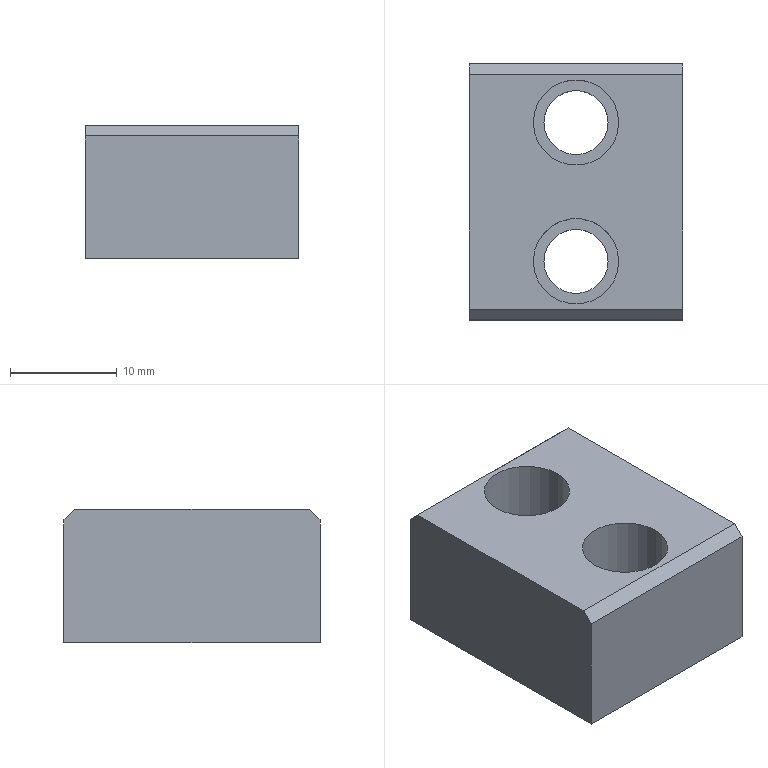Part | STEP file | Ngam kep 12 | 1 solid | 18 faces | box 20 x 24 x 12.5 mm | volume 5009 mm3 | plane 10 | cylinder 8 | commonest cylinder face diameters 6 x4 8 x4
STEP:
#1=CARTESIAN_POINT('',(0.,0.,0.));
#2=DIRECTION('',(0.,0.,1.));
#3=DIRECTION('',(1.,0.,0.));
#4=AXIS2_PLACEMENT_3D('',#1,#2,#3);
#5=CARTESIAN_POINT('',(4.,6.5,0.25));
#6=VERTEX_POINT('',#5);
#7=CARTESIAN_POINT('',(4.,6.5,6.25));
#8=VERTEX_POINT('',#7);
#9=CARTESIAN_POINT('',(4.,6.5,6.25));
#10=DIRECTION('',(0.,0.,1.));
#11=VECTOR('',#10,1.);
#12=LINE('',#9,#11);
#13=CARTESIAN_POINT('',(0.,6.5,6.25));
#14=DIRECTION('',(0.,0.,1.));
#15=DIRECTION('',(1.,0.,0.));
#16=AXIS2_PLACEMENT_3D('',#13,#14,#15);
#17=CYLINDRICAL_SURFACE('',#16,4.);
#18=CARTESIAN_POINT('',(6.283,0.));
#19=DIRECTION('',(0.,1.));
#20=VECTOR('',#19,1.);
#21=LINE('',#18,#20);
#22=(GEOMETRIC_REPRESENTATION_CONTEXT(2)PARAMETRIC_REPRESENTATION_CONTEXT()REPRESENTATION_CONTEXT('',''));
#23=DEFINITIONAL_REPRESENTATION('',(#21),#22);
#24=PCURVE('',#17,#23);
#25=CARTESIAN_POINT('',(0.,6.5,6.25));
#26=DIRECTION('',(0.,0.,1.));
#27=DIRECTION('',(1.,0.,0.));
#28=AXIS2_PLACEMENT_3D('',#25,#26,#27);
#29=CYLINDRICAL_SURFACE('',#28,4.);
#30=CARTESIAN_POINT('',(0.,0.));
#31=DIRECTION('',(0.,1.));
#32=VECTOR('',#31,1.);
#33=LINE('',#30,#32);
#34=(GEOMETRIC_REPRESENTATION_CONTEXT(2)PARAMETRIC_REPRESENTATION_CONTEXT()REPRESENTATION_CONTEXT('',''));
#35=DEFINITIONAL_REPRESENTATION('',(#33),#34);
#36=PCURVE('',#29,#35);
#37=SURFACE_CURVE('',#12,(#24,#36),.PCURVE_S1.);
#38=EDGE_CURVE('',#6,#8,#37,.T.);
#39=ORIENTED_EDGE('',*,*,#38,.T.);
#40=CARTESIAN_POINT('',(-4.,6.5,6.25));
#41=VERTEX_POINT('',#40);
#42=CARTESIAN_POINT('',(0.,6.5,6.25));
#43=DIRECTION('',(0.,0.,1.));
#44=DIRECTION('',(1.,0.,0.));
#45=AXIS2_PLACEMENT_3D('',#42,#43,#44);
#46=CIRCLE('',#45,4.);
#47=CARTESIAN_POINT('',(0.,0.));
#48=DIRECTION('',(1.,0.));
#49=VECTOR('',#48,1.);
#50=LINE('',#47,#49);
#51=(GEOMETRIC_REPRESENTATION_CONTEXT(2)PARAMETRIC_REPRESENTATION_CONTEXT()REPRESENTATION_CONTEXT('',''));
#52=DEFINITIONAL_REPRESENTATION('',(#50),#51);
#53=PCURVE('',#17,#52);
#54=CARTESIAN_POINT('',(0.,0.,6.25));
#55=DIRECTION('',(0.,0.,1.));
#56=DIRECTION('',(1.,0.,0.));
#57=AXIS2_PLACEMENT_3D('',#54,#55,#56);
#58=PLANE('',#57);
#59=CARTESIAN_POINT('',(0.,6.5));
#60=DIRECTION('',(1.,0.));
#61=AXIS2_PLACEMENT_2D('',#59,#60);
#62=CIRCLE('',#61,4.);
#63=(GEOMETRIC_REPRESENTATION_CONTEXT(2)PARAMETRIC_REPRESENTATION_CONTEXT()REPRESENTATION_CONTEXT('',''));
#64=DEFINITIONAL_REPRESENTATION('',(#62),#63);
#65=PCURVE('',#58,#64);
#66=SURFACE_CURVE('',#46,(#53,#65),.PCURVE_S1.);
#67=EDGE_CURVE('',#41,#8,#66,.T.);
#68=ORIENTED_EDGE('',*,*,#67,.F.);
#69=CARTESIAN_POINT('',(-4.,6.5,0.25));
#70=VERTEX_POINT('',#69);
#71=CARTESIAN_POINT('',(-4.,6.5,6.25));
#72=DIRECTION('',(0.,0.,1.));
#73=VECTOR('',#72,1.);
#74=LINE('',#71,#73);
#75=CARTESIAN_POINT('',(3.142,0.));
#76=DIRECTION('',(0.,1.));
#77=VECTOR('',#76,1.);
#78=LINE('',#75,#77);
#79=(GEOMETRIC_REPRESENTATION_CONTEXT(2)PARAMETRIC_REPRESENTATION_CONTEXT()REPRESENTATION_CONTEXT('',''));
#80=DEFINITIONAL_REPRESENTATION('',(#78),#79);
#81=PCURVE('',#17,#80);
#82=CARTESIAN_POINT('',(3.142,0.));
#83=DIRECTION('',(0.,1.));
#84=VECTOR('',#83,1.);
#85=LINE('',#82,#84);
#86=(GEOMETRIC_REPRESENTATION_CONTEXT(2)PARAMETRIC_REPRESENTATION_CONTEXT()REPRESENTATION_CONTEXT('',''));
#87=DEFINITIONAL_REPRESENTATION('',(#85),#86);
#88=PCURVE('',#29,#87);
#89=SURFACE_CURVE('',#74,(#81,#88),.PCURVE_S1.);
#90=EDGE_CURVE('',#70,#41,#89,.T.);
#91=ORIENTED_EDGE('',*,*,#90,.F.);
#92=CARTESIAN_POINT('',(0.,6.5,0.25));
#93=DIRECTION('',(0.,0.,1.));
#94=DIRECTION('',(1.,0.,0.));
#95=AXIS2_PLACEMENT_3D('',#92,#93,#94);
#96=CIRCLE('',#95,4.);
#97=CARTESIAN_POINT('',(0.,-6.));
#98=DIRECTION('',(1.,0.));
#99=VECTOR('',#98,1.);
#100=LINE('',#97,#99);
#101=(GEOMETRIC_REPRESENTATION_CONTEXT(2)PARAMETRIC_REPRESENTATION_CONTEXT()REPRESENTATION_CONTEXT('',''));
#102=DEFINITIONAL_REPRESENTATION('',(#100),#101);
#103=PCURVE('',#17,#102);
#104=CARTESIAN_POINT('',(3.,6.5,0.25));
#105=DIRECTION('',(0.,0.,-1.));
#106=DIRECTION('',(-1.,0.,0.));
#107=AXIS2_PLACEMENT_3D('',#104,#105,#106);
#108=PLANE('',#107);
#109=CARTESIAN_POINT('',(-1.,0.));
#110=CARTESIAN_POINT('',(-1.,6.928));
#111=CARTESIAN_POINT('',(5.,3.464));
#112=CARTESIAN_POINT('',(11.,0.));
#113=CARTESIAN_POINT('',(5.,-3.464));
#114=CARTESIAN_POINT('',(-1.,-6.928));
#115=CARTESIAN_POINT('',(-1.,0.));
#116=(BOUNDED_CURVE()B_SPLINE_CURVE(2,(#109,#110,#111,#112,#113,#114,#115),.UNSPECIFIED.,.T.,.F.)B_SPLINE_CURVE_WITH_KNOTS((1,2,2,2,2,1),(-2.094,0.,2.094,4.189,6.283,8.378),.UNSPECIFIED.)CURVE()GEOMETRIC_REPRESENTATION_ITEM()RATIONAL_B_SPLINE_CURVE((1.,0.5,1.,0.5,1.,0.5,1.))REPRESENTATION_ITEM(''));
#117=(GEOMETRIC_REPRESENTATION_CONTEXT(2)PARAMETRIC_REPRESENTATION_CONTEXT()REPRESENTATION_CONTEXT('',''));
#118=DEFINITIONAL_REPRESENTATION('',(#116),#117);
#119=PCURVE('',#108,#118);
#120=SURFACE_CURVE('',#96,(#103,#119),.PCURVE_S1.);
#121=EDGE_CURVE('',#70,#6,#120,.T.);
#122=ORIENTED_EDGE('',*,*,#121,.T.);
#123=EDGE_LOOP('',(#39,#68,#91,#122));
#124=FACE_BOUND('',#123,.F.);
#125=ADVANCED_FACE('',(#124),#17,.F.);
#126=CARTESIAN_POINT('',(3.,6.5,-6.25));
#127=VERTEX_POINT('',#126);
#128=CARTESIAN_POINT('',(3.,6.5,0.25));
#129=VERTEX_POINT('',#128);
#130=CARTESIAN_POINT('',(3.,6.5,6.25));
#131=DIRECTION('',(0.,0.,1.));
#132=VECTOR('',#131,1.);
#133=LINE('',#130,#132);
#134=CARTESIAN_POINT('',(0.,6.5,6.25));
#135=DIRECTION('',(0.,0.,1.));
#136=DIRECTION('',(1.,0.,0.));
#137=AXIS2_PLACEMENT_3D('',#134,#135,#136);
#138=CYLINDRICAL_SURFACE('',#137,3.);
#139=CARTESIAN_POINT('',(6.283,0.));
#140=DIRECTION('',(0.,1.));
#141=VECTOR('',#140,1.);
#142=LINE('',#139,#141);
#143=(GEOMETRIC_REPRESENTATION_CONTEXT(2)PARAMETRIC_REPRESENTATION_CONTEXT()REPRESENTATION_CONTEXT('',''));
#144=DEFINITIONAL_REPRESENTATION('',(#142),#143);
#145=PCURVE('',#138,#144);
#146=CARTESIAN_POINT('',(0.,6.5,6.25));
#147=DIRECTION('',(0.,0.,1.));
#148=DIRECTION('',(1.,0.,0.));
#149=AXIS2_PLACEMENT_3D('',#146,#147,#148);
#150=CYLINDRICAL_SURFACE('',#149,3.);
#151=CARTESIAN_POINT('',(0.,0.));
#152=DIRECTION('',(0.,1.));
#153=VECTOR('',#152,1.);
#154=LINE('',#151,#153);
#155=(GEOMETRIC_REPRESENTATION_CONTEXT(2)PARAMETRIC_REPRESENTATION_CONTEXT()REPRESENTATION_CONTEXT('',''));
#156=DEFINITIONAL_REPRESENTATION('',(#154),#155);
#157=PCURVE('',#150,#156);
#158=SURFACE_CURVE('',#133,(#145,#157),.PCURVE_S1.);
#159=EDGE_CURVE('',#127,#129,#158,.T.);
#160=ORIENTED_EDGE('',*,*,#159,.T.);
#161=CARTESIAN_POINT('',(-3.,6.5,0.25));
#162=VERTEX_POINT('',#161);
#163=CARTESIAN_POINT('',(0.,6.5,0.25));
#164=DIRECTION('',(0.,0.,1.));
#165=DIRECTION('',(1.,0.,0.));
#166=AXIS2_PLACEMENT_3D('',#163,#164,#165);
#167=CIRCLE('',#166,3.);
#168=CARTESIAN_POINT('',(0.,-6.));
#169=DIRECTION('',(1.,0.));
#170=VECTOR('',#169,1.);
#171=LINE('',#168,#170);
#172=(GEOMETRIC_REPRESENTATION_CONTEXT(2)PARAMETRIC_REPRESENTATION_CONTEXT()REPRESENTATION_CONTEXT('',''));
#173=DEFINITIONAL_REPRESENTATION('',(#171),#172);
#174=PCURVE('',#138,#173);
#175=CARTESIAN_POINT('',(0.,0.));
#176=CARTESIAN_POINT('',(0.,5.196));
#177=CARTESIAN_POINT('',(4.5,2.598));
#178=CARTESIAN_POINT('',(9.,0.));
#179=CARTESIAN_POINT('',(4.5,-2.598));
#180=CARTESIAN_POINT('',(0.,-5.196));
#181=CARTESIAN_POINT('',(0.,0.));
#182=(BOUNDED_CURVE()B_SPLINE_CURVE(2,(#175,#176,#177,#178,#179,#180,#181),.UNSPECIFIED.,.T.,.F.)B_SPLINE_CURVE_WITH_KNOTS((1,2,2,2,2,1),(-2.094,0.,2.094,4.189,6.283,8.378),.UNSPECIFIED.)CURVE()GEOMETRIC_REPRESENTATION_ITEM()RATIONAL_B_SPLINE_CURVE((1.,0.5,1.,0.5,1.,0.5,1.))REPRESENTATION_ITEM(''));
#183=(GEOMETRIC_REPRESENTATION_CONTEXT(2)PARAMETRIC_REPRESENTATION_CONTEXT()REPRESENTATION_CONTEXT('',''));
#184=DEFINITIONAL_REPRESENTATION('',(#182),#183);
#185=PCURVE('',#108,#184);
#186=SURFACE_CURVE('',#167,(#174,#185),.PCURVE_S1.);
#187=EDGE_CURVE('',#162,#129,#186,.T.);
#188=ORIENTED_EDGE('',*,*,#187,.F.);
#189=CARTESIAN_POINT('',(-3.,6.5,-6.25));
#190=VERTEX_POINT('',#189);
#191=CARTESIAN_POINT('',(-3.,6.5,6.25));
#192=DIRECTION('',(0.,0.,1.));
#193=VECTOR('',#192,1.);
#194=LINE('',#191,#193);
#195=CARTESIAN_POINT('',(3.142,0.));
#196=DIRECTION('',(0.,1.));
#197=VECTOR('',#196,1.);
#198=LINE('',#195,#197);
#199=(GEOMETRIC_REPRESENTATION_CONTEXT(2)PARAMETRIC_REPRESENTATION_CONTEXT()REPRESENTATION_CONTEXT('',''));
#200=DEFINITIONAL_REPRESENTATION('',(#198),#199);
#201=PCURVE('',#138,#200);
#202=CARTESIAN_POINT('',(3.142,0.));
#203=DIRECTION('',(0.,1.));
#204=VECTOR('',#203,1.);
#205=LINE('',#202,#204);
#206=(GEOMETRIC_REPRESENTATION_CONTEXT(2)PARAMETRIC_REPRESENTATION_CONTEXT()REPRESENTATION_CONTEXT('',''));
#207=DEFINITIONAL_REPRESENTATION('',(#205),#206);
#208=PCURVE('',#150,#207);
#209=SURFACE_CURVE('',#194,(#201,#208),.PCURVE_S1.);
#210=EDGE_CURVE('',#190,#162,#209,.T.);
#211=ORIENTED_EDGE('',*,*,#210,.F.);
#212=CARTESIAN_POINT('',(0.,6.5,-6.25));
#213=DIRECTION('',(0.,0.,1.));
#214=DIRECTION('',(1.,0.,0.));
#215=AXIS2_PLACEMENT_3D('',#212,#213,#214);
#216=CIRCLE('',#215,3.);
#217=CARTESIAN_POINT('',(0.,-12.5));
#218=DIRECTION('',(1.,0.));
#219=VECTOR('',#218,1.);
#220=LINE('',#217,#219);
#221=(GEOMETRIC_REPRESENTATION_CONTEXT(2)PARAMETRIC_REPRESENTATION_CONTEXT()REPRESENTATION_CONTEXT('',''));
#222=DEFINITIONAL_REPRESENTATION('',(#220),#221);
#223=PCURVE('',#138,#222);
#224=CARTESIAN_POINT('',(0.,0.,-6.25));
#225=DIRECTION('',(0.,0.,1.));
#226=DIRECTION('',(1.,0.,0.));
#227=AXIS2_PLACEMENT_3D('',#224,#225,#226);
#228=PLANE('',#227);
#229=CARTESIAN_POINT('',(0.,6.5));
#230=DIRECTION('',(1.,0.));
#231=AXIS2_PLACEMENT_2D('',#229,#230);
#232=CIRCLE('',#231,3.);
#233=(GEOMETRIC_REPRESENTATION_CONTEXT(2)PARAMETRIC_REPRESENTATION_CONTEXT()REPRESENTATION_CONTEXT('',''));
#234=DEFINITIONAL_REPRESENTATION('',(#232),#233);
#235=PCURVE('',#228,#234);
#236=SURFACE_CURVE('',#216,(#223,#235),.PCURVE_S1.);
#237=EDGE_CURVE('',#190,#127,#236,.T.);
#238=ORIENTED_EDGE('',*,*,#237,.T.);
#239=EDGE_LOOP('',(#160,#188,#211,#238));
#240=FACE_BOUND('',#239,.F.);
#241=ADVANCED_FACE('',(#240),#138,.F.);
#242=CARTESIAN_POINT('',(4.,-6.5,0.25));
#243=VERTEX_POINT('',#242);
#244=CARTESIAN_POINT('',(4.,-6.5,6.25));
#245=VERTEX_POINT('',#244);
#246=CARTESIAN_POINT('',(4.,-6.5,6.25));
#247=DIRECTION('',(0.,0.,1.));
#248=VECTOR('',#247,1.);
#249=LINE('',#246,#248);
#250=CARTESIAN_POINT('',(0.,-6.5,6.25));
#251=DIRECTION('',(0.,0.,1.));
#252=DIRECTION('',(1.,0.,0.));
#253=AXIS2_PLACEMENT_3D('',#250,#251,#252);
#254=CYLINDRICAL_SURFACE('',#253,4.);
#255=CARTESIAN_POINT('',(6.283,0.));
#256=DIRECTION('',(0.,1.));
#257=VECTOR('',#256,1.);
#258=LINE('',#255,#257);
#259=(GEOMETRIC_REPRESENTATION_CONTEXT(2)PARAMETRIC_REPRESENTATION_CONTEXT()REPRESENTATION_CONTEXT('',''));
#260=DEFINITIONAL_REPRESENTATION('',(#258),#259);
#261=PCURVE('',#254,#260);
#262=CARTESIAN_POINT('',(0.,-6.5,6.25));
#263=DIRECTION('',(0.,0.,1.));
#264=DIRECTION('',(1.,0.,0.));
#265=AXIS2_PLACEMENT_3D('',#262,#263,#264);
#266=CYLINDRICAL_SURFACE('',#265,4.);
#267=CARTESIAN_POINT('',(0.,0.));
#268=DIRECTION('',(0.,1.));
#269=VECTOR('',#268,1.);
#270=LINE('',#267,#269);
#271=(GEOMETRIC_REPRESENTATION_CONTEXT(2)PARAMETRIC_REPRESENTATION_CONTEXT()REPRESENTATION_CONTEXT('',''));
#272=DEFINITIONAL_REPRESENTATION('',(#270),#271);
#273=PCURVE('',#266,#272);
#274=SURFACE_CURVE('',#249,(#261,#273),.PCURVE_S1.);
#275=EDGE_CURVE('',#243,#245,#274,.T.);
#276=ORIENTED_EDGE('',*,*,#275,.T.);
#277=CARTESIAN_POINT('',(-4.,-6.5,6.25));
#278=VERTEX_POINT('',#277);
#279=CARTESIAN_POINT('',(0.,-6.5,6.25));
#280=DIRECTION('',(0.,0.,1.));
#281=DIRECTION('',(1.,0.,0.));
#282=AXIS2_PLACEMENT_3D('',#279,#280,#281);
#283=CIRCLE('',#282,4.);
#284=CARTESIAN_POINT('',(0.,0.));
#285=DIRECTION('',(1.,0.));
#286=VECTOR('',#285,1.);
#287=LINE('',#284,#286);
#288=(GEOMETRIC_REPRESENTATION_CONTEXT(2)PARAMETRIC_REPRESENTATION_CONTEXT()REPRESENTATION_CONTEXT('',''));
#289=DEFINITIONAL_REPRESENTATION('',(#287),#288);
#290=PCURVE('',#254,#289);
#291=CARTESIAN_POINT('',(0.,-6.5));
#292=DIRECTION('',(1.,0.));
#293=AXIS2_PLACEMENT_2D('',#291,#292);
#294=CIRCLE('',#293,4.);
#295=(GEOMETRIC_REPRESENTATION_CONTEXT(2)PARAMETRIC_REPRESENTATION_CONTEXT()REPRESENTATION_CONTEXT('',''));
#296=DEFINITIONAL_REPRESENTATION('',(#294),#295);
#297=PCURVE('',#58,#296);
#298=SURFACE_CURVE('',#283,(#290,#297),.PCURVE_S1.);
#299=EDGE_CURVE('',#278,#245,#298,.T.);
#300=ORIENTED_EDGE('',*,*,#299,.F.);
#301=CARTESIAN_POINT('',(-4.,-6.5,0.25));
#302=VERTEX_POINT('',#301);
#303=CARTESIAN_POINT('',(-4.,-6.5,6.25));
#304=DIRECTION('',(0.,0.,1.));
#305=VECTOR('',#304,1.);
#306=LINE('',#303,#305);
#307=CARTESIAN_POINT('',(3.142,0.));
#308=DIRECTION('',(0.,1.));
#309=VECTOR('',#308,1.);
#310=LINE('',#307,#309);
#311=(GEOMETRIC_REPRESENTATION_CONTEXT(2)PARAMETRIC_REPRESENTATION_CONTEXT()REPRESENTATION_CONTEXT('',''));
#312=DEFINITIONAL_REPRESENTATION('',(#310),#311);
#313=PCURVE('',#254,#312);
#314=CARTESIAN_POINT('',(3.142,0.));
#315=DIRECTION('',(0.,1.));
#316=VECTOR('',#315,1.);
#317=LINE('',#314,#316);
#318=(GEOMETRIC_REPRESENTATION_CONTEXT(2)PARAMETRIC_REPRESENTATION_CONTEXT()REPRESENTATION_CONTEXT('',''));
#319=DEFINITIONAL_REPRESENTATION('',(#317),#318);
#320=PCURVE('',#266,#319);
#321=SURFACE_CURVE('',#306,(#313,#320),.PCURVE_S1.);
#322=EDGE_CURVE('',#302,#278,#321,.T.);
#323=ORIENTED_EDGE('',*,*,#322,.F.);
#324=CARTESIAN_POINT('',(0.,-6.5,0.25));
#325=DIRECTION('',(0.,0.,1.));
#326=DIRECTION('',(1.,0.,0.));
#327=AXIS2_PLACEMENT_3D('',#324,#325,#326);
#328=CIRCLE('',#327,4.);
#329=CARTESIAN_POINT('',(0.,-6.));
#330=DIRECTION('',(1.,0.));
#331=VECTOR('',#330,1.);
#332=LINE('',#329,#331);
#333=(GEOMETRIC_REPRESENTATION_CONTEXT(2)PARAMETRIC_REPRESENTATION_CONTEXT()REPRESENTATION_CONTEXT('',''));
#334=DEFINITIONAL_REPRESENTATION('',(#332),#333);
#335=PCURVE('',#254,#334);
#336=CARTESIAN_POINT('',(3.,-6.5,0.25));
#337=DIRECTION('',(0.,0.,-1.));
#338=DIRECTION('',(-1.,0.,0.));
#339=AXIS2_PLACEMENT_3D('',#336,#337,#338);
#340=PLANE('',#339);
#341=CARTESIAN_POINT('',(-1.,0.));
#342=CARTESIAN_POINT('',(-1.,6.928));
#343=CARTESIAN_POINT('',(5.,3.464));
#344=CARTESIAN_POINT('',(11.,0.));
#345=CARTESIAN_POINT('',(5.,-3.464));
#346=CARTESIAN_POINT('',(-1.,-6.928));
#347=CARTESIAN_POINT('',(-1.,0.));
#348=(BOUNDED_CURVE()B_SPLINE_CURVE(2,(#341,#342,#343,#344,#345,#346,#347),.UNSPECIFIED.,.T.,.F.)B_SPLINE_CURVE_WITH_KNOTS((1,2,2,2,2,1),(-2.094,0.,2.094,4.189,6.283,8.378),.UNSPECIFIED.)CURVE()GEOMETRIC_REPRESENTATION_ITEM()RATIONAL_B_SPLINE_CURVE((1.,0.5,1.,0.5,1.,0.5,1.))REPRESENTATION_ITEM(''));
#349=(GEOMETRIC_REPRESENTATION_CONTEXT(2)PARAMETRIC_REPRESENTATION_CONTEXT()REPRESENTATION_CONTEXT('',''));
#350=DEFINITIONAL_REPRESENTATION('',(#348),#349);
#351=PCURVE('',#340,#350);
#352=SURFACE_CURVE('',#328,(#335,#351),.PCURVE_S1.);
#353=EDGE_CURVE('',#302,#243,#352,.T.);
#354=ORIENTED_EDGE('',*,*,#353,.T.);
#355=EDGE_LOOP('',(#276,#300,#323,#354));
#356=FACE_BOUND('',#355,.F.);
#357=ADVANCED_FACE('',(#356),#254,.F.);
#358=CARTESIAN_POINT('',(3.,-6.5,-6.25));
#359=VERTEX_POINT('',#358);
#360=CARTESIAN_POINT('',(3.,-6.5,0.25));
#361=VERTEX_POINT('',#360);
#362=CARTESIAN_POINT('',(3.,-6.5,6.25));
#363=DIRECTION('',(0.,0.,1.));
#364=VECTOR('',#363,1.);
#365=LINE('',#362,#364);
#366=CARTESIAN_POINT('',(0.,-6.5,6.25));
#367=DIRECTION('',(0.,0.,1.));
#368=DIRECTION('',(1.,0.,0.));
#369=AXIS2_PLACEMENT_3D('',#366,#367,#368);
#370=CYLINDRICAL_SURFACE('',#369,3.);
#371=CARTESIAN_POINT('',(6.283,0.));
#372=DIRECTION('',(0.,1.));
#373=VECTOR('',#372,1.);
#374=LINE('',#371,#373);
#375=(GEOMETRIC_REPRESENTATION_CONTEXT(2)PARAMETRIC_REPRESENTATION_CONTEXT()REPRESENTATION_CONTEXT('',''));
#376=DEFINITIONAL_REPRESENTATION('',(#374),#375);
#377=PCURVE('',#370,#376);
#378=CARTESIAN_POINT('',(0.,-6.5,6.25));
#379=DIRECTION('',(0.,0.,1.));
#380=DIRECTION('',(1.,0.,0.));
#381=AXIS2_PLACEMENT_3D('',#378,#379,#380);
#382=CYLINDRICAL_SURFACE('',#381,3.);
#383=CARTESIAN_POINT('',(0.,0.));
#384=DIRECTION('',(0.,1.));
#385=VECTOR('',#384,1.);
#386=LINE('',#383,#385);
#387=(GEOMETRIC_REPRESENTATION_CONTEXT(2)PARAMETRIC_REPRESENTATION_CONTEXT()REPRESENTATION_CONTEXT('',''));
#388=DEFINITIONAL_REPRESENTATION('',(#386),#387);
#389=PCURVE('',#382,#388);
#390=SURFACE_CURVE('',#365,(#377,#389),.PCURVE_S1.);
#391=EDGE_CURVE('',#359,#361,#390,.T.);
#392=ORIENTED_EDGE('',*,*,#391,.T.);
#393=CARTESIAN_POINT('',(-3.,-6.5,0.25));
#394=VERTEX_POINT('',#393);
#395=CARTESIAN_POINT('',(0.,-6.5,0.25));
#396=DIRECTION('',(0.,0.,1.));
#397=DIRECTION('',(1.,0.,0.));
#398=AXIS2_PLACEMENT_3D('',#395,#396,#397);
#399=CIRCLE('',#398,3.);
#400=CARTESIAN_POINT('',(0.,-6.));
#401=DIRECTION('',(1.,0.));
#402=VECTOR('',#401,1.);
#403=LINE('',#400,#402);
#404=(GEOMETRIC_REPRESENTATION_CONTEXT(2)PARAMETRIC_REPRESENTATION_CONTEXT()REPRESENTATION_CONTEXT('',''));
#405=DEFINITIONAL_REPRESENTATION('',(#403),#404);
#406=PCURVE('',#370,#405);
#407=CARTESIAN_POINT('',(0.,0.));
#408=CARTESIAN_POINT('',(0.,5.196));
#409=CARTESIAN_POINT('',(4.5,2.598));
#410=CARTESIAN_POINT('',(9.,0.));
#411=CARTESIAN_POINT('',(4.5,-2.598));
#412=CARTESIAN_POINT('',(0.,-5.196));
#413=CARTESIAN_POINT('',(0.,0.));
#414=(BOUNDED_CURVE()B_SPLINE_CURVE(2,(#407,#408,#409,#410,#411,#412,#413),.UNSPECIFIED.,.T.,.F.)B_SPLINE_CURVE_WITH_KNOTS((1,2,2,2,2,1),(-2.094,0.,2.094,4.189,6.283,8.378),.UNSPECIFIED.)CURVE()GEOMETRIC_REPRESENTATION_ITEM()RATIONAL_B_SPLINE_CURVE((1.,0.5,1.,0.5,1.,0.5,1.))REPRESENTATION_ITEM(''));
#415=(GEOMETRIC_REPRESENTATION_CONTEXT(2)PARAMETRIC_REPRESENTATION_CONTEXT()REPRESENTATION_CONTEXT('',''));
#416=DEFINITIONAL_REPRESENTATION('',(#414),#415);
#417=PCURVE('',#340,#416);
#418=SURFACE_CURVE('',#399,(#406,#417),.PCURVE_S1.);
#419=EDGE_CURVE('',#394,#361,#418,.T.);
#420=ORIENTED_EDGE('',*,*,#419,.F.);
#421=CARTESIAN_POINT('',(-3.,-6.5,-6.25));
#422=VERTEX_POINT('',#421);
#423=CARTESIAN_POINT('',(-3.,-6.5,6.25));
#424=DIRECTION('',(0.,0.,1.));
#425=VECTOR('',#424,1.);
#426=LINE('',#423,#425);
#427=CARTESIAN_POINT('',(3.142,0.));
#428=DIRECTION('',(0.,1.));
#429=VECTOR('',#428,1.);
#430=LINE('',#427,#429);
#431=(GEOMETRIC_REPRESENTATION_CONTEXT(2)PARAMETRIC_REPRESENTATION_CONTEXT()REPRESENTATION_CONTEXT('',''));
#432=DEFINITIONAL_REPRESENTATION('',(#430),#431);
#433=PCURVE('',#370,#432);
#434=CARTESIAN_POINT('',(3.142,0.));
#435=DIRECTION('',(0.,1.));
#436=VECTOR('',#435,1.);
#437=LINE('',#434,#436);
#438=(GEOMETRIC_REPRESENTATION_CONTEXT(2)PARAMETRIC_REPRESENTATION_CONTEXT()REPRESENTATION_CONTEXT('',''));
#439=DEFINITIONAL_REPRESENTATION('',(#437),#438);
#440=PCURVE('',#382,#439);
#441=SURFACE_CURVE('',#426,(#433,#440),.PCURVE_S1.);
#442=EDGE_CURVE('',#422,#394,#441,.T.);
#443=ORIENTED_EDGE('',*,*,#442,.F.);
#444=CARTESIAN_POINT('',(0.,-6.5,-6.25));
#445=DIRECTION('',(0.,0.,1.));
#446=DIRECTION('',(1.,0.,0.));
#447=AXIS2_PLACEMENT_3D('',#444,#445,#446);
#448=CIRCLE('',#447,3.);
#449=CARTESIAN_POINT('',(0.,-12.5));
#450=DIRECTION('',(1.,0.));
#451=VECTOR('',#450,1.);
#452=LINE('',#449,#451);
#453=(GEOMETRIC_REPRESENTATION_CONTEXT(2)PARAMETRIC_REPRESENTATION_CONTEXT()REPRESENTATION_CONTEXT('',''));
#454=DEFINITIONAL_REPRESENTATION('',(#452),#453);
#455=PCURVE('',#370,#454);
#456=CARTESIAN_POINT('',(0.,-6.5));
#457=DIRECTION('',(1.,0.));
#458=AXIS2_PLACEMENT_2D('',#456,#457);
#459=CIRCLE('',#458,3.);
#460=(GEOMETRIC_REPRESENTATION_CONTEXT(2)PARAMETRIC_REPRESENTATION_CONTEXT()REPRESENTATION_CONTEXT('',''));
#461=DEFINITIONAL_REPRESENTATION('',(#459),#460);
#462=PCURVE('',#228,#461);
#463=SURFACE_CURVE('',#448,(#455,#462),.PCURVE_S1.);
#464=EDGE_CURVE('',#422,#359,#463,.T.);
#465=ORIENTED_EDGE('',*,*,#464,.T.);
#466=EDGE_LOOP('',(#392,#420,#443,#465));
#467=FACE_BOUND('',#466,.F.);
#468=ADVANCED_FACE('',(#467),#370,.F.);
#469=CARTESIAN_POINT('',(-10.,-12.,5.25));
#470=VERTEX_POINT('',#469);
#471=CARTESIAN_POINT('',(-10.,-12.,-6.25));
#472=VERTEX_POINT('',#471);
#473=CARTESIAN_POINT('',(-10.,-12.,6.25));
#474=DIRECTION('',(0.,0.,-1.));
#475=VECTOR('',#474,1.);
#476=LINE('',#473,#475);
#477=CARTESIAN_POINT('',(-10.,12.,6.25));
#478=DIRECTION('',(1.,0.,0.));
#479=DIRECTION('',(0.,1.,0.));
#480=AXIS2_PLACEMENT_3D('',#477,#478,#479);
#481=PLANE('',#480);
#482=CARTESIAN_POINT('',(-24.,0.));
#483=DIRECTION('',(0.,-1.));
#484=VECTOR('',#483,1.);
#485=LINE('',#482,#484);
#486=(GEOMETRIC_REPRESENTATION_CONTEXT(2)PARAMETRIC_REPRESENTATION_CONTEXT()REPRESENTATION_CONTEXT('',''));
#487=DEFINITIONAL_REPRESENTATION('',(#485),#486);
#488=PCURVE('',#481,#487);
#489=CARTESIAN_POINT('',(-10.,-12.,6.25));
#490=DIRECTION('',(0.,1.,0.));
#491=DIRECTION('',(0.,0.,1.));
#492=AXIS2_PLACEMENT_3D('',#489,#490,#491);
#493=PLANE('',#492);
#494=CARTESIAN_POINT('',(0.,0.));
#495=DIRECTION('',(-1.,0.));
#496=VECTOR('',#495,1.);
#497=LINE('',#494,#496);
#498=(GEOMETRIC_REPRESENTATION_CONTEXT(2)PARAMETRIC_REPRESENTATION_CONTEXT()REPRESENTATION_CONTEXT('',''));
#499=DEFINITIONAL_REPRESENTATION('',(#497),#498);
#500=PCURVE('',#493,#499);
#501=SURFACE_CURVE('',#476,(#488,#500),.PCURVE_S1.);
#502=EDGE_CURVE('',#470,#472,#501,.T.);
#503=ORIENTED_EDGE('',*,*,#502,.F.);
#504=CARTESIAN_POINT('',(-10.,-11.,6.25));
#505=VERTEX_POINT('',#504);
#506=CARTESIAN_POINT('',(-10.,-11.,6.25));
#507=DIRECTION('',(0.,0.7071,0.7071));
#508=VECTOR('',#507,1.);
#509=LINE('',#506,#508);
#510=CARTESIAN_POINT('',(-23.,0.));
#511=DIRECTION('',(0.7071,0.7071));
#512=VECTOR('',#511,1.);
#513=LINE('',#510,#512);
#514=(GEOMETRIC_REPRESENTATION_CONTEXT(2)PARAMETRIC_REPRESENTATION_CONTEXT()REPRESENTATION_CONTEXT('',''));
#515=DEFINITIONAL_REPRESENTATION('',(#513),#514);
#516=PCURVE('',#481,#515);
#517=CARTESIAN_POINT('',(0.,-11.,6.25));
#518=DIRECTION('',(0.,-0.7071,0.7071));
#519=DIRECTION('',(-1.,0.,0.));
#520=AXIS2_PLACEMENT_3D('',#517,#518,#519);
#521=PLANE('',#520);
#522=CARTESIAN_POINT('',(10.,0.));
#523=DIRECTION('',(0.,-1.));
#524=VECTOR('',#523,1.);
#525=LINE('',#522,#524);
#526=(GEOMETRIC_REPRESENTATION_CONTEXT(2)PARAMETRIC_REPRESENTATION_CONTEXT()REPRESENTATION_CONTEXT('',''));
#527=DEFINITIONAL_REPRESENTATION('',(#525),#526);
#528=PCURVE('',#521,#527);
#529=SURFACE_CURVE('',#509,(#516,#528),.PCURVE_S1.);
#530=EDGE_CURVE('',#470,#505,#529,.T.);
#531=ORIENTED_EDGE('',*,*,#530,.T.);
#532=CARTESIAN_POINT('',(-10.,11.,6.25));
#533=VERTEX_POINT('',#532);
#534=CARTESIAN_POINT('',(-10.,12.,6.25));
#535=DIRECTION('',(0.,-1.,0.));
#536=VECTOR('',#535,1.);
#537=LINE('',#534,#536);
#538=CARTESIAN_POINT('',(0.,0.));
#539=DIRECTION('',(-1.,0.));
#540=VECTOR('',#539,1.);
#541=LINE('',#538,#540);
#542=(GEOMETRIC_REPRESENTATION_CONTEXT(2)PARAMETRIC_REPRESENTATION_CONTEXT()REPRESENTATION_CONTEXT('',''));
#543=DEFINITIONAL_REPRESENTATION('',(#541),#542);
#544=PCURVE('',#481,#543);
#545=CARTESIAN_POINT('',(-10.,12.));
#546=DIRECTION('',(0.,-1.));
#547=VECTOR('',#546,1.);
#548=LINE('',#545,#547);
#549=(GEOMETRIC_REPRESENTATION_CONTEXT(2)PARAMETRIC_REPRESENTATION_CONTEXT()REPRESENTATION_CONTEXT('',''));
#550=DEFINITIONAL_REPRESENTATION('',(#548),#549);
#551=PCURVE('',#58,#550);
#552=SURFACE_CURVE('',#537,(#544,#551),.PCURVE_S1.);
#553=EDGE_CURVE('',#533,#505,#552,.T.);
#554=ORIENTED_EDGE('',*,*,#553,.F.);
#555=CARTESIAN_POINT('',(-10.,12.,5.25));
#556=VERTEX_POINT('',#555);
#557=CARTESIAN_POINT('',(-10.,11.,6.25));
#558=DIRECTION('',(0.,0.7071,-0.7071));
#559=VECTOR('',#558,1.);
#560=LINE('',#557,#559);
#561=CARTESIAN_POINT('',(-1.,0.));
#562=DIRECTION('',(0.7071,-0.7071));
#563=VECTOR('',#562,1.);
#564=LINE('',#561,#563);
#565=(GEOMETRIC_REPRESENTATION_CONTEXT(2)PARAMETRIC_REPRESENTATION_CONTEXT()REPRESENTATION_CONTEXT('',''));
#566=DEFINITIONAL_REPRESENTATION('',(#564),#565);
#567=PCURVE('',#481,#566);
#568=CARTESIAN_POINT('',(0.,11.,6.25));
#569=DIRECTION('',(0.,0.7071,0.7071));
#570=DIRECTION('',(1.,0.,0.));
#571=AXIS2_PLACEMENT_3D('',#568,#569,#570);
#572=PLANE('',#571);
#573=CARTESIAN_POINT('',(-10.,0.));
#574=DIRECTION('',(0.,1.));
#575=VECTOR('',#574,1.);
#576=LINE('',#573,#575);
#577=(GEOMETRIC_REPRESENTATION_CONTEXT(2)PARAMETRIC_REPRESENTATION_CONTEXT()REPRESENTATION_CONTEXT('',''));
#578=DEFINITIONAL_REPRESENTATION('',(#576),#577);
#579=PCURVE('',#572,#578);
#580=SURFACE_CURVE('',#560,(#567,#579),.PCURVE_S1.);
#581=EDGE_CURVE('',#533,#556,#580,.T.);
#582=ORIENTED_EDGE('',*,*,#581,.T.);
#583=CARTESIAN_POINT('',(-10.,12.,-6.25));
#584=VERTEX_POINT('',#583);
#585=CARTESIAN_POINT('',(-10.,12.,6.25));
#586=DIRECTION('',(0.,0.,-1.));
#587=VECTOR('',#586,1.);
#588=LINE('',#585,#587);
#589=CARTESIAN_POINT('',(0.,0.));
#590=DIRECTION('',(0.,-1.));
#591=VECTOR('',#590,1.);
#592=LINE('',#589,#591);
#593=(GEOMETRIC_REPRESENTATION_CONTEXT(2)PARAMETRIC_REPRESENTATION_CONTEXT()REPRESENTATION_CONTEXT('',''));
#594=DEFINITIONAL_REPRESENTATION('',(#592),#593);
#595=PCURVE('',#481,#594);
#596=CARTESIAN_POINT('',(-10.,12.,6.25));
#597=DIRECTION('',(0.,-1.,0.));
#598=DIRECTION('',(0.,0.,-1.));
#599=AXIS2_PLACEMENT_3D('',#596,#597,#598);
#600=PLANE('',#599);
#601=CARTESIAN_POINT('',(0.,0.));
#602=DIRECTION('',(1.,0.));
#603=VECTOR('',#602,1.);
#604=LINE('',#601,#603);
#605=(GEOMETRIC_REPRESENTATION_CONTEXT(2)PARAMETRIC_REPRESENTATION_CONTEXT()REPRESENTATION_CONTEXT('',''));
#606=DEFINITIONAL_REPRESENTATION('',(#604),#605);
#607=PCURVE('',#600,#606);
#608=SURFACE_CURVE('',#588,(#595,#607),.PCURVE_S1.);
#609=EDGE_CURVE('',#556,#584,#608,.T.);
#610=ORIENTED_EDGE('',*,*,#609,.T.);
#611=CARTESIAN_POINT('',(-10.,12.,-6.25));
#612=DIRECTION('',(0.,-1.,0.));
#613=VECTOR('',#612,1.);
#614=LINE('',#611,#613);
#615=CARTESIAN_POINT('',(0.,-12.5));
#616=DIRECTION('',(-1.,0.));
#617=VECTOR('',#616,1.);
#618=LINE('',#615,#617);
#619=(GEOMETRIC_REPRESENTATION_CONTEXT(2)PARAMETRIC_REPRESENTATION_CONTEXT()REPRESENTATION_CONTEXT('',''));
#620=DEFINITIONAL_REPRESENTATION('',(#618),#619);
#621=PCURVE('',#481,#620);
#622=CARTESIAN_POINT('',(-10.,12.));
#623=DIRECTION('',(0.,-1.));
#624=VECTOR('',#623,1.);
#625=LINE('',#622,#624);
#626=(GEOMETRIC_REPRESENTATION_CONTEXT(2)PARAMETRIC_REPRESENTATION_CONTEXT()REPRESENTATION_CONTEXT('',''));
#627=DEFINITIONAL_REPRESENTATION('',(#625),#626);
#628=PCURVE('',#228,#627);
#629=SURFACE_CURVE('',#614,(#621,#628),.PCURVE_S1.);
#630=EDGE_CURVE('',#584,#472,#629,.T.);
#631=ORIENTED_EDGE('',*,*,#630,.T.);
#632=EDGE_LOOP('',(#503,#531,#554,#582,#610,#631));
#633=FACE_BOUND('',#632,.T.);
#634=ADVANCED_FACE('',(#633),#481,.F.);
#635=CARTESIAN_POINT('',(10.,-12.,5.25));
#636=VERTEX_POINT('',#635);
#637=CARTESIAN_POINT('',(10.,-12.,-6.25));
#638=VERTEX_POINT('',#637);
#639=CARTESIAN_POINT('',(10.,-12.,6.25));
#640=DIRECTION('',(0.,0.,-1.));
#641=VECTOR('',#640,1.);
#642=LINE('',#639,#641);
#643=CARTESIAN_POINT('',(0.,20.));
#644=DIRECTION('',(-1.,0.));
#645=VECTOR('',#644,1.);
#646=LINE('',#643,#645);
#647=(GEOMETRIC_REPRESENTATION_CONTEXT(2)PARAMETRIC_REPRESENTATION_CONTEXT()REPRESENTATION_CONTEXT('',''));
#648=DEFINITIONAL_REPRESENTATION('',(#646),#647);
#649=PCURVE('',#493,#648);
#650=CARTESIAN_POINT('',(10.,12.,6.25));
#651=DIRECTION('',(-1.,0.,0.));
#652=DIRECTION('',(0.,-1.,0.));
#653=AXIS2_PLACEMENT_3D('',#650,#651,#652);
#654=PLANE('',#653);
#655=CARTESIAN_POINT('',(24.,0.));
#656=DIRECTION('',(0.,-1.));
#657=VECTOR('',#656,1.);
#658=LINE('',#655,#657);
#659=(GEOMETRIC_REPRESENTATION_CONTEXT(2)PARAMETRIC_REPRESENTATION_CONTEXT()REPRESENTATION_CONTEXT('',''));
#660=DEFINITIONAL_REPRESENTATION('',(#658),#659);
#661=PCURVE('',#654,#660);
#662=SURFACE_CURVE('',#642,(#649,#661),.PCURVE_S1.);
#663=EDGE_CURVE('',#636,#638,#662,.T.);
#664=ORIENTED_EDGE('',*,*,#663,.F.);
#665=CARTESIAN_POINT('',(-10.,-12.,5.25));
#666=DIRECTION('',(-1.,0.,0.));
#667=VECTOR('',#666,1.);
#668=LINE('',#665,#667);
#669=CARTESIAN_POINT('',(-1.,0.));
#670=DIRECTION('',(0.,-1.));
#671=VECTOR('',#670,1.);
#672=LINE('',#669,#671);
#673=(GEOMETRIC_REPRESENTATION_CONTEXT(2)PARAMETRIC_REPRESENTATION_CONTEXT()REPRESENTATION_CONTEXT('',''));
#674=DEFINITIONAL_REPRESENTATION('',(#672),#673);
#675=PCURVE('',#493,#674);
#676=CARTESIAN_POINT('',(10.,1.414));
#677=DIRECTION('',(1.,0.));
#678=VECTOR('',#677,1.);
#679=LINE('',#676,#678);
#680=(GEOMETRIC_REPRESENTATION_CONTEXT(2)PARAMETRIC_REPRESENTATION_CONTEXT()REPRESENTATION_CONTEXT('',''));
#681=DEFINITIONAL_REPRESENTATION('',(#679),#680);
#682=PCURVE('',#521,#681);
#683=SURFACE_CURVE('',#668,(#675,#682),.PCURVE_S1.);
#684=EDGE_CURVE('',#636,#470,#683,.T.);
#685=ORIENTED_EDGE('',*,*,#684,.T.);
#686=ORIENTED_EDGE('',*,*,#502,.T.);
#687=CARTESIAN_POINT('',(-10.,-12.,-6.25));
#688=DIRECTION('',(1.,0.,0.));
#689=VECTOR('',#688,1.);
#690=LINE('',#687,#689);
#691=CARTESIAN_POINT('',(-12.5,0.));
#692=DIRECTION('',(0.,1.));
#693=VECTOR('',#692,1.);
#694=LINE('',#691,#693);
#695=(GEOMETRIC_REPRESENTATION_CONTEXT(2)PARAMETRIC_REPRESENTATION_CONTEXT()REPRESENTATION_CONTEXT('',''));
#696=DEFINITIONAL_REPRESENTATION('',(#694),#695);
#697=PCURVE('',#493,#696);
#698=CARTESIAN_POINT('',(-10.,-12.));
#699=DIRECTION('',(1.,0.));
#700=VECTOR('',#699,1.);
#701=LINE('',#698,#700);
#702=(GEOMETRIC_REPRESENTATION_CONTEXT(2)PARAMETRIC_REPRESENTATION_CONTEXT()REPRESENTATION_CONTEXT('',''));
#703=DEFINITIONAL_REPRESENTATION('',(#701),#702);
#704=PCURVE('',#228,#703);
#705=SURFACE_CURVE('',#690,(#697,#704),.PCURVE_S1.);
#706=EDGE_CURVE('',#472,#638,#705,.T.);
#707=ORIENTED_EDGE('',*,*,#706,.T.);
#708=EDGE_LOOP('',(#664,#685,#686,#707));
#709=FACE_BOUND('',#708,.T.);
#710=ADVANCED_FACE('',(#709),#493,.F.);
#711=CARTESIAN_POINT('',(10.,-11.,6.25));
#712=VERTEX_POINT('',#711);
#713=CARTESIAN_POINT('',(10.,11.,6.25));
#714=VERTEX_POINT('',#713);
#715=CARTESIAN_POINT('',(10.,12.,6.25));
#716=DIRECTION('',(0.,1.,0.));
#717=VECTOR('',#716,1.);
#718=LINE('',#715,#717);
#719=CARTESIAN_POINT('',(0.,0.));
#720=DIRECTION('',(-1.,0.));
#721=VECTOR('',#720,1.);
#722=LINE('',#719,#721);
#723=(GEOMETRIC_REPRESENTATION_CONTEXT(2)PARAMETRIC_REPRESENTATION_CONTEXT()REPRESENTATION_CONTEXT('',''));
#724=DEFINITIONAL_REPRESENTATION('',(#722),#723);
#725=PCURVE('',#654,#724);
#726=CARTESIAN_POINT('',(10.,12.));
#727=DIRECTION('',(0.,1.));
#728=VECTOR('',#727,1.);
#729=LINE('',#726,#728);
#730=(GEOMETRIC_REPRESENTATION_CONTEXT(2)PARAMETRIC_REPRESENTATION_CONTEXT()REPRESENTATION_CONTEXT('',''));
#731=DEFINITIONAL_REPRESENTATION('',(#729),#730);
#732=PCURVE('',#58,#731);
#733=SURFACE_CURVE('',#718,(#725,#732),.PCURVE_S1.);
#734=EDGE_CURVE('',#712,#714,#733,.T.);
#735=ORIENTED_EDGE('',*,*,#734,.F.);
#736=CARTESIAN_POINT('',(10.,-11.,6.25));
#737=DIRECTION('',(0.,-0.7071,-0.7071));
#738=VECTOR('',#737,1.);
#739=LINE('',#736,#738);
#740=CARTESIAN_POINT('',(23.,0.));
#741=DIRECTION('',(0.7071,-0.7071));
#742=VECTOR('',#741,1.);
#743=LINE('',#740,#742);
#744=(GEOMETRIC_REPRESENTATION_CONTEXT(2)PARAMETRIC_REPRESENTATION_CONTEXT()REPRESENTATION_CONTEXT('',''));
#745=DEFINITIONAL_REPRESENTATION('',(#743),#744);
#746=PCURVE('',#654,#745);
#747=CARTESIAN_POINT('',(-10.,0.));
#748=DIRECTION('',(0.,1.));
#749=VECTOR('',#748,1.);
#750=LINE('',#747,#749);
#751=(GEOMETRIC_REPRESENTATION_CONTEXT(2)PARAMETRIC_REPRESENTATION_CONTEXT()REPRESENTATION_CONTEXT('',''));
#752=DEFINITIONAL_REPRESENTATION('',(#750),#751);
#753=PCURVE('',#521,#752);
#754=SURFACE_CURVE('',#739,(#746,#753),.PCURVE_S1.);
#755=EDGE_CURVE('',#712,#636,#754,.T.);
#756=ORIENTED_EDGE('',*,*,#755,.T.);
#757=ORIENTED_EDGE('',*,*,#663,.T.);
#758=CARTESIAN_POINT('',(10.,12.,-6.25));
#759=VERTEX_POINT('',#758);
#760=CARTESIAN_POINT('',(10.,12.,-6.25));
#761=DIRECTION('',(0.,1.,0.));
#762=VECTOR('',#761,1.);
#763=LINE('',#760,#762);
#764=CARTESIAN_POINT('',(0.,-12.5));
#765=DIRECTION('',(-1.,0.));
#766=VECTOR('',#765,1.);
#767=LINE('',#764,#766);
#768=(GEOMETRIC_REPRESENTATION_CONTEXT(2)PARAMETRIC_REPRESENTATION_CONTEXT()REPRESENTATION_CONTEXT('',''));
#769=DEFINITIONAL_REPRESENTATION('',(#767),#768);
#770=PCURVE('',#654,#769);
#771=CARTESIAN_POINT('',(10.,12.));
#772=DIRECTION('',(0.,1.));
#773=VECTOR('',#772,1.);
#774=LINE('',#771,#773);
#775=(GEOMETRIC_REPRESENTATION_CONTEXT(2)PARAMETRIC_REPRESENTATION_CONTEXT()REPRESENTATION_CONTEXT('',''));
#776=DEFINITIONAL_REPRESENTATION('',(#774),#775);
#777=PCURVE('',#228,#776);
#778=SURFACE_CURVE('',#763,(#770,#777),.PCURVE_S1.);
#779=EDGE_CURVE('',#638,#759,#778,.T.);
#780=ORIENTED_EDGE('',*,*,#779,.T.);
#781=CARTESIAN_POINT('',(10.,12.,5.25));
#782=VERTEX_POINT('',#781);
#783=CARTESIAN_POINT('',(10.,12.,6.25));
#784=DIRECTION('',(0.,0.,-1.));
#785=VECTOR('',#784,1.);
#786=LINE('',#783,#785);
#787=CARTESIAN_POINT('',(0.,0.));
#788=DIRECTION('',(0.,-1.));
#789=VECTOR('',#788,1.);
#790=LINE('',#787,#789);
#791=(GEOMETRIC_REPRESENTATION_CONTEXT(2)PARAMETRIC_REPRESENTATION_CONTEXT()REPRESENTATION_CONTEXT('',''));
#792=DEFINITIONAL_REPRESENTATION('',(#790),#791);
#793=PCURVE('',#654,#792);
#794=CARTESIAN_POINT('',(0.,20.));
#795=DIRECTION('',(1.,0.));
#796=VECTOR('',#795,1.);
#797=LINE('',#794,#796);
#798=(GEOMETRIC_REPRESENTATION_CONTEXT(2)PARAMETRIC_REPRESENTATION_CONTEXT()REPRESENTATION_CONTEXT('',''));
#799=DEFINITIONAL_REPRESENTATION('',(#797),#798);
#800=PCURVE('',#600,#799);
#801=SURFACE_CURVE('',#786,(#793,#800),.PCURVE_S1.);
#802=EDGE_CURVE('',#782,#759,#801,.T.);
#803=ORIENTED_EDGE('',*,*,#802,.F.);
#804=CARTESIAN_POINT('',(10.,11.,6.25));
#805=DIRECTION('',(0.,-0.7071,0.7071));
#806=VECTOR('',#805,1.);
#807=LINE('',#804,#806);
#808=CARTESIAN_POINT('',(1.,0.));
#809=DIRECTION('',(0.7071,0.7071));
#810=VECTOR('',#809,1.);
#811=LINE('',#808,#810);
#812=(GEOMETRIC_REPRESENTATION_CONTEXT(2)PARAMETRIC_REPRESENTATION_CONTEXT()REPRESENTATION_CONTEXT('',''));
#813=DEFINITIONAL_REPRESENTATION('',(#811),#812);
#814=PCURVE('',#654,#813);
#815=CARTESIAN_POINT('',(10.,0.));
#816=DIRECTION('',(0.,-1.));
#817=VECTOR('',#816,1.);
#818=LINE('',#815,#817);
#819=(GEOMETRIC_REPRESENTATION_CONTEXT(2)PARAMETRIC_REPRESENTATION_CONTEXT()REPRESENTATION_CONTEXT('',''));
#820=DEFINITIONAL_REPRESENTATION('',(#818),#819);
#821=PCURVE('',#572,#820);
#822=SURFACE_CURVE('',#807,(#814,#821),.PCURVE_S1.);
#823=EDGE_CURVE('',#782,#714,#822,.T.);
#824=ORIENTED_EDGE('',*,*,#823,.T.);
#825=EDGE_LOOP('',(#735,#756,#757,#780,#803,#824));
#826=FACE_BOUND('',#825,.T.);
#827=ADVANCED_FACE('',(#826),#654,.F.);
#828=ORIENTED_EDGE('',*,*,#609,.F.);
#829=CARTESIAN_POINT('',(10.,12.,5.25));
#830=DIRECTION('',(1.,0.,0.));
#831=VECTOR('',#830,1.);
#832=LINE('',#829,#831);
#833=CARTESIAN_POINT('',(1.,20.));
#834=DIRECTION('',(0.,1.));
#835=VECTOR('',#834,1.);
#836=LINE('',#833,#835);
#837=(GEOMETRIC_REPRESENTATION_CONTEXT(2)PARAMETRIC_REPRESENTATION_CONTEXT()REPRESENTATION_CONTEXT('',''));
#838=DEFINITIONAL_REPRESENTATION('',(#836),#837);
#839=PCURVE('',#600,#838);
#840=CARTESIAN_POINT('',(10.,1.414));
#841=DIRECTION('',(1.,0.));
#842=VECTOR('',#841,1.);
#843=LINE('',#840,#842);
#844=(GEOMETRIC_REPRESENTATION_CONTEXT(2)PARAMETRIC_REPRESENTATION_CONTEXT()REPRESENTATION_CONTEXT('',''));
#845=DEFINITIONAL_REPRESENTATION('',(#843),#844);
#846=PCURVE('',#572,#845);
#847=SURFACE_CURVE('',#832,(#839,#846),.PCURVE_S1.);
#848=EDGE_CURVE('',#556,#782,#847,.T.);
#849=ORIENTED_EDGE('',*,*,#848,.T.);
#850=ORIENTED_EDGE('',*,*,#802,.T.);
#851=CARTESIAN_POINT('',(-10.,12.,-6.25));
#852=DIRECTION('',(-1.,0.,0.));
#853=VECTOR('',#852,1.);
#854=LINE('',#851,#853);
#855=CARTESIAN_POINT('',(12.5,0.));
#856=DIRECTION('',(0.,-1.));
#857=VECTOR('',#856,1.);
#858=LINE('',#855,#857);
#859=(GEOMETRIC_REPRESENTATION_CONTEXT(2)PARAMETRIC_REPRESENTATION_CONTEXT()REPRESENTATION_CONTEXT('',''));
#860=DEFINITIONAL_REPRESENTATION('',(#858),#859);
#861=PCURVE('',#600,#860);
#862=CARTESIAN_POINT('',(-10.,12.));
#863=DIRECTION('',(-1.,0.));
#864=VECTOR('',#863,1.);
#865=LINE('',#862,#864);
#866=(GEOMETRIC_REPRESENTATION_CONTEXT(2)PARAMETRIC_REPRESENTATION_CONTEXT()REPRESENTATION_CONTEXT('',''));
#867=DEFINITIONAL_REPRESENTATION('',(#865),#866);
#868=PCURVE('',#228,#867);
#869=SURFACE_CURVE('',#854,(#861,#868),.PCURVE_S1.);
#870=EDGE_CURVE('',#759,#584,#869,.T.);
#871=ORIENTED_EDGE('',*,*,#870,.T.);
#872=EDGE_LOOP('',(#828,#849,#850,#871));
#873=FACE_BOUND('',#872,.T.);
#874=ADVANCED_FACE('',(#873),#600,.F.);
#875=CARTESIAN_POINT('',(0.,6.5,6.25));
#876=DIRECTION('',(0.,0.,1.));
#877=DIRECTION('',(1.,0.,0.));
#878=AXIS2_PLACEMENT_3D('',#875,#876,#877);
#879=CIRCLE('',#878,4.);
#880=CARTESIAN_POINT('',(0.,6.5));
#881=DIRECTION('',(1.,0.));
#882=AXIS2_PLACEMENT_2D('',#880,#881);
#883=CIRCLE('',#882,4.);
#884=(GEOMETRIC_REPRESENTATION_CONTEXT(2)PARAMETRIC_REPRESENTATION_CONTEXT()REPRESENTATION_CONTEXT('',''));
#885=DEFINITIONAL_REPRESENTATION('',(#883),#884);
#886=PCURVE('',#58,#885);
#887=CARTESIAN_POINT('',(0.,0.));
#888=DIRECTION('',(1.,0.));
#889=VECTOR('',#888,1.);
#890=LINE('',#887,#889);
#891=(GEOMETRIC_REPRESENTATION_CONTEXT(2)PARAMETRIC_REPRESENTATION_CONTEXT()REPRESENTATION_CONTEXT('',''));
#892=DEFINITIONAL_REPRESENTATION('',(#890),#891);
#893=PCURVE('',#29,#892);
#894=SURFACE_CURVE('',#879,(#886,#893),.PCURVE_S1.);
#895=EDGE_CURVE('',#8,#41,#894,.T.);
#896=ORIENTED_EDGE('',*,*,#895,.F.);
#897=ORIENTED_EDGE('',*,*,#67,.F.);
#898=EDGE_LOOP('',(#896,#897));
#899=FACE_BOUND('',#898,.T.);
#900=CARTESIAN_POINT('',(0.,-6.5,6.25));
#901=DIRECTION('',(0.,0.,1.));
#902=DIRECTION('',(1.,0.,0.));
#903=AXIS2_PLACEMENT_3D('',#900,#901,#902);
#904=CIRCLE('',#903,4.);
#905=CARTESIAN_POINT('',(0.,-6.5));
#906=DIRECTION('',(1.,0.));
#907=AXIS2_PLACEMENT_2D('',#905,#906);
#908=CIRCLE('',#907,4.);
#909=(GEOMETRIC_REPRESENTATION_CONTEXT(2)PARAMETRIC_REPRESENTATION_CONTEXT()REPRESENTATION_CONTEXT('',''));
#910=DEFINITIONAL_REPRESENTATION('',(#908),#909);
#911=PCURVE('',#58,#910);
#912=CARTESIAN_POINT('',(0.,0.));
#913=DIRECTION('',(1.,0.));
#914=VECTOR('',#913,1.);
#915=LINE('',#912,#914);
#916=(GEOMETRIC_REPRESENTATION_CONTEXT(2)PARAMETRIC_REPRESENTATION_CONTEXT()REPRESENTATION_CONTEXT('',''));
#917=DEFINITIONAL_REPRESENTATION('',(#915),#916);
#918=PCURVE('',#266,#917);
#919=SURFACE_CURVE('',#904,(#911,#918),.PCURVE_S1.);
#920=EDGE_CURVE('',#245,#278,#919,.T.);
#921=ORIENTED_EDGE('',*,*,#920,.F.);
#922=ORIENTED_EDGE('',*,*,#299,.F.);
#923=EDGE_LOOP('',(#921,#922));
#924=FACE_BOUND('',#923,.T.);
#925=ORIENTED_EDGE('',*,*,#553,.T.);
#926=CARTESIAN_POINT('',(10.,-11.,6.25));
#927=DIRECTION('',(1.,0.,0.));
#928=VECTOR('',#927,1.);
#929=LINE('',#926,#928);
#930=CARTESIAN_POINT('',(10.,-11.));
#931=DIRECTION('',(1.,0.));
#932=VECTOR('',#931,1.);
#933=LINE('',#930,#932);
#934=(GEOMETRIC_REPRESENTATION_CONTEXT(2)PARAMETRIC_REPRESENTATION_CONTEXT()REPRESENTATION_CONTEXT('',''));
#935=DEFINITIONAL_REPRESENTATION('',(#933),#934);
#936=PCURVE('',#58,#935);
#937=CARTESIAN_POINT('',(-10.,0.));
#938=DIRECTION('',(-1.,0.));
#939=VECTOR('',#938,1.);
#940=LINE('',#937,#939);
#941=(GEOMETRIC_REPRESENTATION_CONTEXT(2)PARAMETRIC_REPRESENTATION_CONTEXT()REPRESENTATION_CONTEXT('',''));
#942=DEFINITIONAL_REPRESENTATION('',(#940),#941);
#943=PCURVE('',#521,#942);
#944=SURFACE_CURVE('',#929,(#936,#943),.PCURVE_S1.);
#945=EDGE_CURVE('',#505,#712,#944,.T.);
#946=ORIENTED_EDGE('',*,*,#945,.T.);
#947=ORIENTED_EDGE('',*,*,#734,.T.);
#948=CARTESIAN_POINT('',(-10.,11.,6.25));
#949=DIRECTION('',(-1.,0.,0.));
#950=VECTOR('',#949,1.);
#951=LINE('',#948,#950);
#952=CARTESIAN_POINT('',(-10.,11.));
#953=DIRECTION('',(-1.,0.));
#954=VECTOR('',#953,1.);
#955=LINE('',#952,#954);
#956=(GEOMETRIC_REPRESENTATION_CONTEXT(2)PARAMETRIC_REPRESENTATION_CONTEXT()REPRESENTATION_CONTEXT('',''));
#957=DEFINITIONAL_REPRESENTATION('',(#955),#956);
#958=PCURVE('',#58,#957);
#959=CARTESIAN_POINT('',(-10.,0.));
#960=DIRECTION('',(-1.,0.));
#961=VECTOR('',#960,1.);
#962=LINE('',#959,#961);
#963=(GEOMETRIC_REPRESENTATION_CONTEXT(2)PARAMETRIC_REPRESENTATION_CONTEXT()REPRESENTATION_CONTEXT('',''));
#964=DEFINITIONAL_REPRESENTATION('',(#962),#963);
#965=PCURVE('',#572,#964);
#966=SURFACE_CURVE('',#951,(#958,#965),.PCURVE_S1.);
#967=EDGE_CURVE('',#714,#533,#966,.T.);
#968=ORIENTED_EDGE('',*,*,#967,.T.);
#969=EDGE_LOOP('',(#925,#946,#947,#968));
#970=FACE_BOUND('',#969,.T.);
#971=ADVANCED_FACE('',(#899,#924,#970),#58,.T.);
#972=CARTESIAN_POINT('',(0.,6.5,-6.25));
#973=DIRECTION('',(0.,0.,1.));
#974=DIRECTION('',(1.,0.,0.));
#975=AXIS2_PLACEMENT_3D('',#972,#973,#974);
#976=CIRCLE('',#975,3.);
#977=CARTESIAN_POINT('',(0.,6.5));
#978=DIRECTION('',(1.,0.));
#979=AXIS2_PLACEMENT_2D('',#977,#978);
#980=CIRCLE('',#979,3.);
#981=(GEOMETRIC_REPRESENTATION_CONTEXT(2)PARAMETRIC_REPRESENTATION_CONTEXT()REPRESENTATION_CONTEXT('',''));
#982=DEFINITIONAL_REPRESENTATION('',(#980),#981);
#983=PCURVE('',#228,#982);
#984=CARTESIAN_POINT('',(0.,-12.5));
#985=DIRECTION('',(1.,0.));
#986=VECTOR('',#985,1.);
#987=LINE('',#984,#986);
#988=(GEOMETRIC_REPRESENTATION_CONTEXT(2)PARAMETRIC_REPRESENTATION_CONTEXT()REPRESENTATION_CONTEXT('',''));
#989=DEFINITIONAL_REPRESENTATION('',(#987),#988);
#990=PCURVE('',#150,#989);
#991=SURFACE_CURVE('',#976,(#983,#990),.PCURVE_S1.);
#992=EDGE_CURVE('',#127,#190,#991,.T.);
#993=ORIENTED_EDGE('',*,*,#992,.T.);
#994=ORIENTED_EDGE('',*,*,#237,.T.);
#995=EDGE_LOOP('',(#993,#994));
#996=FACE_BOUND('',#995,.T.);
#997=CARTESIAN_POINT('',(0.,-6.5,-6.25));
#998=DIRECTION('',(0.,0.,1.));
#999=DIRECTION('',(1.,0.,0.));
#1000=AXIS2_PLACEMENT_3D('',#997,#998,#999);
#1001=CIRCLE('',#1000,3.);
#1002=CARTESIAN_POINT('',(0.,-6.5));
#1003=DIRECTION('',(1.,0.));
#1004=AXIS2_PLACEMENT_2D('',#1002,#1003);
#1005=CIRCLE('',#1004,3.);
#1006=(GEOMETRIC_REPRESENTATION_CONTEXT(2)PARAMETRIC_REPRESENTATION_CONTEXT()REPRESENTATION_CONTEXT('',''));
#1007=DEFINITIONAL_REPRESENTATION('',(#1005),#1006);
#1008=PCURVE('',#228,#1007);
#1009=CARTESIAN_POINT('',(0.,-12.5));
#1010=DIRECTION('',(1.,0.));
#1011=VECTOR('',#1010,1.);
#1012=LINE('',#1009,#1011);
#1013=(GEOMETRIC_REPRESENTATION_CONTEXT(2)PARAMETRIC_REPRESENTATION_CONTEXT()REPRESENTATION_CONTEXT('',''));
#1014=DEFINITIONAL_REPRESENTATION('',(#1012),#1013);
#1015=PCURVE('',#382,#1014);
#1016=SURFACE_CURVE('',#1001,(#1008,#1015),.PCURVE_S1.);
#1017=EDGE_CURVE('',#359,#422,#1016,.T.);
#1018=ORIENTED_EDGE('',*,*,#1017,.T.);
#1019=ORIENTED_EDGE('',*,*,#464,.T.);
#1020=EDGE_LOOP('',(#1018,#1019));
#1021=FACE_BOUND('',#1020,.T.);
#1022=ORIENTED_EDGE('',*,*,#630,.F.);
#1023=ORIENTED_EDGE('',*,*,#870,.F.);
#1024=ORIENTED_EDGE('',*,*,#779,.F.);
#1025=ORIENTED_EDGE('',*,*,#706,.F.);
#1026=EDGE_LOOP('',(#1022,#1023,#1024,#1025));
#1027=FACE_BOUND('',#1026,.T.);
#1028=ADVANCED_FACE('',(#996,#1021,#1027),#228,.F.);
#1029=CARTESIAN_POINT('',(0.,-6.5,0.25));
#1030=DIRECTION('',(0.,0.,1.));
#1031=DIRECTION('',(1.,0.,0.));
#1032=AXIS2_PLACEMENT_3D('',#1029,#1030,#1031);
#1033=CIRCLE('',#1032,3.);
#1034=CARTESIAN_POINT('',(0.,-6.));
#1035=DIRECTION('',(1.,0.));
#1036=VECTOR('',#1035,1.);
#1037=LINE('',#1034,#1036);
#1038=(GEOMETRIC_REPRESENTATION_CONTEXT(2)PARAMETRIC_REPRESENTATION_CONTEXT()REPRESENTATION_CONTEXT('',''));
#1039=DEFINITIONAL_REPRESENTATION('',(#1037),#1038);
#1040=PCURVE('',#382,#1039);
#1041=CARTESIAN_POINT('',(0.,0.));
#1042=CARTESIAN_POINT('',(0.,5.196));
#1043=CARTESIAN_POINT('',(4.5,2.598));
#1044=CARTESIAN_POINT('',(9.,0.));
#1045=CARTESIAN_POINT('',(4.5,-2.598));
#1046=CARTESIAN_POINT('',(0.,-5.196));
#1047=CARTESIAN_POINT('',(0.,0.));
#1048=(BOUNDED_CURVE()B_SPLINE_CURVE(2,(#1041,#1042,#1043,#1044,#1045,#1046,#1047),.UNSPECIFIED.,.T.,.F.)B_SPLINE_CURVE_WITH_KNOTS((1,2,2,2,2,1),(-2.094,0.,2.094,4.189,6.283,8.378),.UNSPECIFIED.)CURVE()GEOMETRIC_REPRESENTATION_ITEM()RATIONAL_B_SPLINE_CURVE((1.,0.5,1.,0.5,1.,0.5,1.))REPRESENTATION_ITEM(''));
#1049=(GEOMETRIC_REPRESENTATION_CONTEXT(2)PARAMETRIC_REPRESENTATION_CONTEXT()REPRESENTATION_CONTEXT('',''));
#1050=DEFINITIONAL_REPRESENTATION('',(#1048),#1049);
#1051=PCURVE('',#340,#1050);
#1052=SURFACE_CURVE('',#1033,(#1040,#1051),.PCURVE_S1.);
#1053=EDGE_CURVE('',#361,#394,#1052,.T.);
#1054=ORIENTED_EDGE('',*,*,#1053,.F.);
#1055=ORIENTED_EDGE('',*,*,#391,.F.);
#1056=ORIENTED_EDGE('',*,*,#1017,.T.);
#1057=ORIENTED_EDGE('',*,*,#442,.T.);
#1058=EDGE_LOOP('',(#1054,#1055,#1056,#1057));
#1059=FACE_BOUND('',#1058,.F.);
#1060=ADVANCED_FACE('',(#1059),#382,.F.);
#1061=ORIENTED_EDGE('',*,*,#1053,.F.);
#1062=ORIENTED_EDGE('',*,*,#419,.F.);
#1063=EDGE_LOOP('',(#1061,#1062));
#1064=FACE_BOUND('',#1063,.T.);
#1065=CARTESIAN_POINT('',(0.,-6.5,0.25));
#1066=DIRECTION('',(0.,0.,1.));
#1067=DIRECTION('',(1.,0.,0.));
#1068=AXIS2_PLACEMENT_3D('',#1065,#1066,#1067);
#1069=CIRCLE('',#1068,4.);
#1070=CARTESIAN_POINT('',(-1.,0.));
#1071=CARTESIAN_POINT('',(-1.,6.928));
#1072=CARTESIAN_POINT('',(5.,3.464));
#1073=CARTESIAN_POINT('',(11.,0.));
#1074=CARTESIAN_POINT('',(5.,-3.464));
#1075=CARTESIAN_POINT('',(-1.,-6.928));
#1076=CARTESIAN_POINT('',(-1.,0.));
#1077=(BOUNDED_CURVE()B_SPLINE_CURVE(2,(#1070,#1071,#1072,#1073,#1074,#1075,#1076),.UNSPECIFIED.,.T.,.F.)B_SPLINE_CURVE_WITH_KNOTS((1,2,2,2,2,1),(-2.094,0.,2.094,4.189,6.283,8.378),.UNSPECIFIED.)CURVE()GEOMETRIC_REPRESENTATION_ITEM()RATIONAL_B_SPLINE_CURVE((1.,0.5,1.,0.5,1.,0.5,1.))REPRESENTATION_ITEM(''));
#1078=(GEOMETRIC_REPRESENTATION_CONTEXT(2)PARAMETRIC_REPRESENTATION_CONTEXT()REPRESENTATION_CONTEXT('',''));
#1079=DEFINITIONAL_REPRESENTATION('',(#1077),#1078);
#1080=PCURVE('',#340,#1079);
#1081=CARTESIAN_POINT('',(0.,-6.));
#1082=DIRECTION('',(1.,0.));
#1083=VECTOR('',#1082,1.);
#1084=LINE('',#1081,#1083);
#1085=(GEOMETRIC_REPRESENTATION_CONTEXT(2)PARAMETRIC_REPRESENTATION_CONTEXT()REPRESENTATION_CONTEXT('',''));
#1086=DEFINITIONAL_REPRESENTATION('',(#1084),#1085);
#1087=PCURVE('',#266,#1086);
#1088=SURFACE_CURVE('',#1069,(#1080,#1087),.PCURVE_S1.);
#1089=EDGE_CURVE('',#243,#302,#1088,.T.);
#1090=ORIENTED_EDGE('',*,*,#1089,.T.);
#1091=ORIENTED_EDGE('',*,*,#353,.T.);
#1092=EDGE_LOOP('',(#1090,#1091));
#1093=FACE_BOUND('',#1092,.T.);
#1094=ADVANCED_FACE('',(#1064,#1093),#340,.F.);
#1095=ORIENTED_EDGE('',*,*,#920,.F.);
#1096=ORIENTED_EDGE('',*,*,#275,.F.);
#1097=ORIENTED_EDGE('',*,*,#1089,.T.);
#1098=ORIENTED_EDGE('',*,*,#322,.T.);
#1099=EDGE_LOOP('',(#1095,#1096,#1097,#1098));
#1100=FACE_BOUND('',#1099,.F.);
#1101=ADVANCED_FACE('',(#1100),#266,.F.);
#1102=CARTESIAN_POINT('',(0.,6.5,0.25));
#1103=DIRECTION('',(0.,0.,1.));
#1104=DIRECTION('',(1.,0.,0.));
#1105=AXIS2_PLACEMENT_3D('',#1102,#1103,#1104);
#1106=CIRCLE('',#1105,3.);
#1107=CARTESIAN_POINT('',(0.,-6.));
#1108=DIRECTION('',(1.,0.));
#1109=VECTOR('',#1108,1.);
#1110=LINE('',#1107,#1109);
#1111=(GEOMETRIC_REPRESENTATION_CONTEXT(2)PARAMETRIC_REPRESENTATION_CONTEXT()REPRESENTATION_CONTEXT('',''));
#1112=DEFINITIONAL_REPRESENTATION('',(#1110),#1111);
#1113=PCURVE('',#150,#1112);
#1114=CARTESIAN_POINT('',(0.,0.));
#1115=CARTESIAN_POINT('',(0.,5.196));
#1116=CARTESIAN_POINT('',(4.5,2.598));
#1117=CARTESIAN_POINT('',(9.,0.));
#1118=CARTESIAN_POINT('',(4.5,-2.598));
#1119=CARTESIAN_POINT('',(0.,-5.196));
#1120=CARTESIAN_POINT('',(0.,0.));
#1121=(BOUNDED_CURVE()B_SPLINE_CURVE(2,(#1114,#1115,#1116,#1117,#1118,#1119,#1120),.UNSPECIFIED.,.T.,.F.)B_SPLINE_CURVE_WITH_KNOTS((1,2,2,2,2,1),(-2.094,0.,2.094,4.189,6.283,8.378),.UNSPECIFIED.)CURVE()GEOMETRIC_REPRESENTATION_ITEM()RATIONAL_B_SPLINE_CURVE((1.,0.5,1.,0.5,1.,0.5,1.))REPRESENTATION_ITEM(''));
#1122=(GEOMETRIC_REPRESENTATION_CONTEXT(2)PARAMETRIC_REPRESENTATION_CONTEXT()REPRESENTATION_CONTEXT('',''));
#1123=DEFINITIONAL_REPRESENTATION('',(#1121),#1122);
#1124=PCURVE('',#108,#1123);
#1125=SURFACE_CURVE('',#1106,(#1113,#1124),.PCURVE_S1.);
#1126=EDGE_CURVE('',#129,#162,#1125,.T.);
#1127=ORIENTED_EDGE('',*,*,#1126,.F.);
#1128=ORIENTED_EDGE('',*,*,#159,.F.);
#1129=ORIENTED_EDGE('',*,*,#992,.T.);
#1130=ORIENTED_EDGE('',*,*,#210,.T.);
#1131=EDGE_LOOP('',(#1127,#1128,#1129,#1130));
#1132=FACE_BOUND('',#1131,.F.);
#1133=ADVANCED_FACE('',(#1132),#150,.F.);
#1134=ORIENTED_EDGE('',*,*,#1126,.F.);
#1135=ORIENTED_EDGE('',*,*,#187,.F.);
#1136=EDGE_LOOP('',(#1134,#1135));
#1137=FACE_BOUND('',#1136,.T.);
#1138=CARTESIAN_POINT('',(0.,6.5,0.25));
#1139=DIRECTION('',(0.,0.,1.));
#1140=DIRECTION('',(1.,0.,0.));
#1141=AXIS2_PLACEMENT_3D('',#1138,#1139,#1140);
#1142=CIRCLE('',#1141,4.);
#1143=CARTESIAN_POINT('',(-1.,0.));
#1144=CARTESIAN_POINT('',(-1.,6.928));
#1145=CARTESIAN_POINT('',(5.,3.464));
#1146=CARTESIAN_POINT('',(11.,0.));
#1147=CARTESIAN_POINT('',(5.,-3.464));
#1148=CARTESIAN_POINT('',(-1.,-6.928));
#1149=CARTESIAN_POINT('',(-1.,0.));
#1150=(BOUNDED_CURVE()B_SPLINE_CURVE(2,(#1143,#1144,#1145,#1146,#1147,#1148,#1149),.UNSPECIFIED.,.T.,.F.)B_SPLINE_CURVE_WITH_KNOTS((1,2,2,2,2,1),(-2.094,0.,2.094,4.189,6.283,8.378),.UNSPECIFIED.)CURVE()GEOMETRIC_REPRESENTATION_ITEM()RATIONAL_B_SPLINE_CURVE((1.,0.5,1.,0.5,1.,0.5,1.))REPRESENTATION_ITEM(''));
#1151=(GEOMETRIC_REPRESENTATION_CONTEXT(2)PARAMETRIC_REPRESENTATION_CONTEXT()REPRESENTATION_CONTEXT('',''));
#1152=DEFINITIONAL_REPRESENTATION('',(#1150),#1151);
#1153=PCURVE('',#108,#1152);
#1154=CARTESIAN_POINT('',(0.,-6.));
#1155=DIRECTION('',(1.,0.));
#1156=VECTOR('',#1155,1.);
#1157=LINE('',#1154,#1156);
#1158=(GEOMETRIC_REPRESENTATION_CONTEXT(2)PARAMETRIC_REPRESENTATION_CONTEXT()REPRESENTATION_CONTEXT('',''));
#1159=DEFINITIONAL_REPRESENTATION('',(#1157),#1158);
#1160=PCURVE('',#29,#1159);
#1161=SURFACE_CURVE('',#1142,(#1153,#1160),.PCURVE_S1.);
#1162=EDGE_CURVE('',#6,#70,#1161,.T.);
#1163=ORIENTED_EDGE('',*,*,#1162,.T.);
#1164=ORIENTED_EDGE('',*,*,#121,.T.);
#1165=EDGE_LOOP('',(#1163,#1164));
#1166=FACE_BOUND('',#1165,.T.);
#1167=ADVANCED_FACE('',(#1137,#1166),#108,.F.);
#1168=ORIENTED_EDGE('',*,*,#895,.F.);
#1169=ORIENTED_EDGE('',*,*,#38,.F.);
#1170=ORIENTED_EDGE('',*,*,#1162,.T.);
#1171=ORIENTED_EDGE('',*,*,#90,.T.);
#1172=EDGE_LOOP('',(#1168,#1169,#1170,#1171));
#1173=FACE_BOUND('',#1172,.F.);
#1174=ADVANCED_FACE('',(#1173),#29,.F.);
#1175=ORIENTED_EDGE('',*,*,#530,.F.);
#1176=ORIENTED_EDGE('',*,*,#684,.F.);
#1177=ORIENTED_EDGE('',*,*,#755,.F.);
#1178=ORIENTED_EDGE('',*,*,#945,.F.);
#1179=EDGE_LOOP('',(#1175,#1176,#1177,#1178));
#1180=FACE_BOUND('',#1179,.T.);
#1181=ADVANCED_FACE('',(#1180),#521,.T.);
#1182=ORIENTED_EDGE('',*,*,#823,.F.);
#1183=ORIENTED_EDGE('',*,*,#848,.F.);
#1184=ORIENTED_EDGE('',*,*,#581,.F.);
#1185=ORIENTED_EDGE('',*,*,#967,.F.);
#1186=EDGE_LOOP('',(#1182,#1183,#1184,#1185));
#1187=FACE_BOUND('',#1186,.T.);
#1188=ADVANCED_FACE('',(#1187),#572,.T.);
#1189=CLOSED_SHELL('',(#125,#241,#357,#468,#634,#710,#827,#874,#971,#1028,#1060,#1094,#1101,#1133,#1167,#1174,#1181,#1188));
#1190=MANIFOLD_SOLID_BREP('',#1189);
#1191=(LENGTH_UNIT()NAMED_UNIT(*)SI_UNIT(.MILLI.,.METRE.));
#1192=UNCERTAINTY_MEASURE_WITH_UNIT(LENGTH_MEASURE(0.0000001),#1191,'','');
#1193=(NAMED_UNIT(*)PLANE_ANGLE_UNIT()SI_UNIT($,.RADIAN.));
#1194=(NAMED_UNIT(*)SI_UNIT($,.STERADIAN.)SOLID_ANGLE_UNIT());
#1195=(GEOMETRIC_REPRESENTATION_CONTEXT(3)GLOBAL_UNCERTAINTY_ASSIGNED_CONTEXT((#1192))GLOBAL_UNIT_ASSIGNED_CONTEXT((#1191,#1193,#1194))REPRESENTATION_CONTEXT('',''));
#1196=ADVANCED_BREP_SHAPE_REPRESENTATION('',(#4,#1190),#1195);